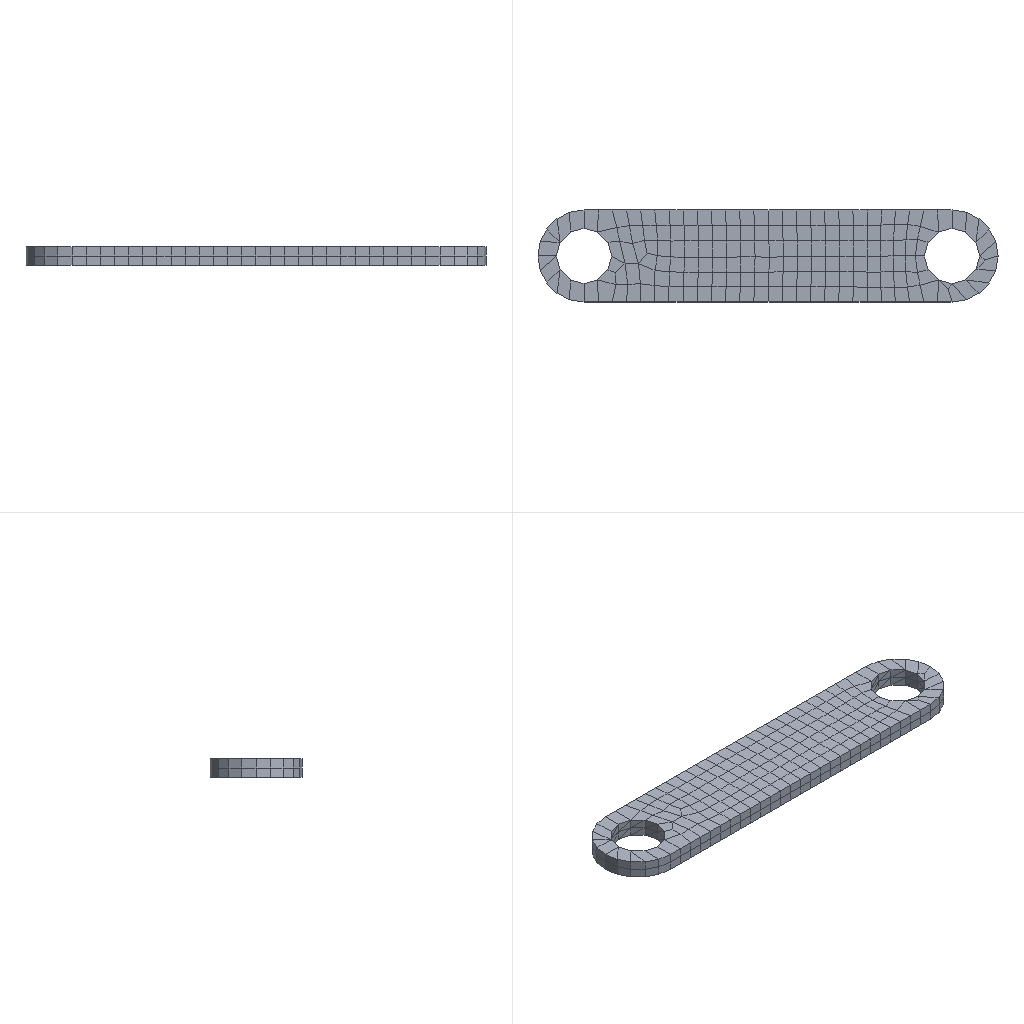Simulation study | ansys workbench
Set-up summary:
category,name,step,type,value,unit,region
solver,ansys_workbench
units,mm-N-s-tonne (MPa),,stated,"/units,MPA"
analysis,LS1,,transient
load_step,LS1,LS1,transient,nsubst=100; time=1
mesh,nodes,,,2205
mesh,elements,,,384
element_type,SOLID186,,,336
element_type,CONTA174,,,48
material,Structural Steel,,E,200000,tonne s^-2 mm^-1
material,Structural Steel,,nu,0.3
material,Structural Steel,,density,7.85e-09,tonne mm^-3
material,Structural Steel,,conductivity,60.5,tonne mm s^-3 C^-1
material,Structural Steel,,specific_heat,4.34e+08,mm^2 s^-2 C^-1
material,Structural Steel,,cte,1.2e-05,C^-1
material,Structural Steel,,permeability,10000
material,Structural Steel,,resistivity,0.00017,ohm mm
contact,contact 1,,bonded (always),element=CONTA174
contact,contact 2,,bonded (always),element=CONTA174
gap,no loads/excitations found in deck
Ansys APDL input file, long lists of numbers shortened:
/batch
/config,noeldb,1     ! force off writing results to database
*get,_wallstrt,active,,time,wall
! ANSYS input file written by Workbench version 2023 R2
! File used for geometry attach:
/title,wbnew--Transient (A5)
! ****** Begin Custom Load Command Snippet ******
/COM, ACT Extensions:
/COM,     LSDYNA, 2023.2
/COM,/COM,     ANSYSMotion, 2023.2
/COM,
! ****** End   Custom Load Command Snippet ******
*DIM,_wb_ProjectScratch_dir,string,248
_wb_ProjectScratch_dir(1) = ''
*DIM,_wb_SolverFiles_dir,string,248
_wb_SolverFiles_dir(1) = ''
*DIM,_wb_userfiles_dir,string,248
_wb_userfiles_dir(1) = ''
/com,--- Data in consistent NMM units. See Solving Units in the help system for more information.
/units,MPA
/nopr
/wb,file,start              !  signify a WB generated input file
/prep7
! Turn off shape checking because checks already performed inside WB mesher.
! See help system for more information.
SHPP,OFF,,NOWARN
/nolist
etcon,set             ! allow ANSYS to choose best KEYOP's for 180x elements, resets any applicable keyopt to MAPDL defaults
/com,*********** Nodes for the whole assembly ***********
nblock,3,,2416
(1i9,3e20.9e3)
        1    -2.448881254E+01     2.152807781E+00     1.630000025E+02
! (2196 more lines like these left out)
-1
/com,*********** Nodes for all Remote Points ***********
nblock,3
(1i9,3e20.9e3)
     2198    -3.448881218E+01     2.152807741E+00     1.630000025E+02
! (7 more lines like these left out)
-1
/wb,elem,start            !  set before creation of elements
/com,*********** Elements for Body 1 "crank" ***********
/com,*********** Send Body as a Rigid Body ***********
et,1,21
keyo,1,2,1             ! Moments of inertia in nodal coordinates
keyo,1,3,0         ! 3D Mass With Rotary Intertia
r,1,3.48526103262952e-006,3.48526103262952e-006,3.48526103262952e-006,3.29793436009623e-005,1.97766587972307e-004,2.28423576723811e-004
local,11,0,-24.489,2.153,163.,0.,0.,0.
nrot,1
csys,0
mat,1
real,1
type,1
en,865,1
/com,*********** Elements for Body 2 "rod" ***********
et,2,186
keyo,2,2,1          ! set full integration on SOLID186
eblock,19,solid,,336
(19i9)
        2        2        2        2        0        0        0        0       20        0        1        8      590      489      516      225      608      514      515
! (671 more lines like these left out)
-1
/com,*********** Elements for Body 3 "sliding" ***********
/com,*********** Send Body as a Rigid Body ***********
et,3,21
keyo,3,2,1             ! Moments of inertia in nodal coordinates
keyo,3,3,0         ! 3D Mass With Rotary Intertia
r,3,1.81689295804776e-006,1.81689295804776e-006,1.81689295804776e-006,2.6747344778675e-005,2.67473433929451e-005,5.22819186247149e-005
local,11,0,25.511,2.153,163.,0.,0.,0.
nrot,2197
csys,0
mat,3
real,3
type,3
en,866,2197
/wb,elem,end               !  done creating elements
/com,*********** Send User Defined Coordinate System(s) ***********
local,12,0,-34.489,2.153,163.,-180.,0.,-180.
local,13,0,-14.489,2.153,163.,-180.,0.,-180.
local,14,0,25.511,2.153,165.,0.,0.,0.
local,15,0,31.511,2.153,163.,0.,0.,0.
csys,0
toffst,273.15,  ! Temperature offset from absolute zero
/com,*********** Set Reference Temperature ***********
tref,22.
/wb,mat,start              !  starting to send materials
/com,*********** Send Materials ***********
Temperature = 'TEMP' ! Temperature
MP,DENS,1,7.85e-09,	! tonne mm^-3
MP,ALPX,1,1.2e-05,	! C^-1
MP,C,1,434000000,	! mm^2 s^-2 C^-1
MP,KXX,1,60.5,	! tonne mm s^-3 C^-1
MP,RSVX,1,0.00017,	! ohm mm
MP,EX,1,200000,	! tonne s^-2 mm^-1
MP,NUXY,1,0.3,
MP,MURX,1,10000,
Temperature = 'TEMP' ! Temperature
MP,DENS,2,7.85e-09,	! tonne mm^-3
MP,ALPX,2,1.2e-05,	! C^-1
MP,C,2,434000000,	! mm^2 s^-2 C^-1
MP,KXX,2,60.5,	! tonne mm s^-3 C^-1
MP,RSVX,2,0.00017,	! ohm mm
MP,EX,2,200000,	! tonne s^-2 mm^-1
MP,NUXY,2,0.3,
MP,MURX,2,10000,
Temperature = 'TEMP' ! Temperature
MP,DENS,3,7.85e-09,	! tonne mm^-3
MP,ALPX,3,1.2e-05,	! C^-1
MP,C,3,434000000,	! mm^2 s^-2 C^-1
MP,KXX,3,60.5,	! tonne mm s^-3 C^-1
MP,RSVX,3,0.00017,	! ohm mm
MP,EX,3,200000,	! tonne s^-2 mm^-1
MP,NUXY,3,0.3,
MP,MURX,3,10000,
/wb,mat,end                !  done sending materials
!************************* Model Summary ********************
!crank,	Structural Steel,	matid,	1
!rod,	Structural Steel,	matid,	2
!sliding,	Structural Steel,	matid,	3
!************************* End Model Summary ********************
! get the diagonal of the bounding box. Needed later for other things
*get,_xmin,node,,mnloc,x
*get,_ymin,node,,mnloc,y
*get,_zmin,node,,mnloc,z
*get,_xmax,node,,mxloc,x
*get,_ymax,node,,mxloc,y
*get,_zmax,node,,mxloc,z
_ASMDIAG=(_xmax-_xmin)*(_xmax-_xmin)+(_ymax-_ymin)*(_ymax-_ymin)+(_zmax-_zmin)*(_zmax-_zmin)
_ASMDIAG=SQRT(_ASMDIAG)
/wb,contact,start          !  starting to send contact
/wb,contact,end            !  done creating contacts
/golist
/wb,load,start             !  starting to send loads
/com,*********** Create Remote Point "Internal Remote Point 2" ***********
! -------- Remote Point Used by "Revolute - Ground To crank" --------
! ********* Create Contact to Connect To Rigid Body Mass Node ***********
*set,tid,4
*set,cid,4
et,tid,170
keyo,tid,2,1           ! Set MPC target element and not fix pilot
keyo,tid,4,0           ! Create CE's for all DOFs
type,tid
mat ,cid
real,cid
tshape,pilo
en,879,1
tshape
! ********* End of Create Contact to Connect To Rigid Body Mass Node ***********
*set,_npilot,2199
_npilot49=_npilot
mat,4
real,4
type,4
en,880,1,2199
csys,12
nrot,2199
csys,0
/com,*********** Create Remote Point "Internal Remote Point 3" ***********
! -------- Remote Point Used by "Revolute - crank To rod" --------
*set,_npilot,2200
_npilot55=_npilot
mat,4
real,4
type,4
en,881,1,2200
csys,13
nrot,2200
csys,0
/com,*********** Create Remote Point "Internal Remote Point 4" ***********
! -------- Remote Point Used by "Revolute - crank To rod" --------
*set,tid,6
*set,cid,5
et,cid,174
et,tid,170
keyo,tid,2,1               ! Don't fix the pilot node
keyo,tid,4,0               ! Activate all DOF's due to large deformation
keyo,cid,12,5              ! Bonded Contact
keyo,cid,4,2               ! Rigid CERIG style load
keyo,cid,2,2               ! MPC style contact
eblock,10,,,24
(15i9)
      882        5        5        5        0      611      623      347      357     2163     1647     1646     1679
! (23 more lines like these left out)
-1
*set,_npilot,2201
_npilot56=_npilot
type,tid
mat ,cid
real,cid
tshape,pilo
en,906,_npilot
tshape
csys,13
nrot,2201
csys,0
/com,*********** Create Remote Point "Internal Remote Point 5" ***********
! -------- Remote Point Used by "Revolute - rod To sliding" --------
*set,tid,8
*set,cid,7
et,cid,174
et,tid,170
keyo,tid,2,1               ! Don't fix the pilot node
keyo,tid,4,0               ! Activate all DOF's due to large deformation
keyo,cid,12,5              ! Bonded Contact
keyo,cid,4,2               ! Rigid CERIG style load
keyo,cid,2,2               ! MPC style contact
eblock,10,,,24
(15i9)
      907        7        7        7        0      587      599      359      369     2127     1685     1683     1713
! (23 more lines like these left out)
-1
*set,_npilot,2202
_npilot63=_npilot
type,tid
mat ,cid
real,cid
tshape,pilo
en,931,_npilot
tshape
/com,*********** Create Remote Point "Internal Remote Point 6" ***********
! -------- Remote Point Used by "Revolute - rod To sliding" --------
! ********* Create Contact to Connect To Rigid Body Mass Node ***********
*set,tid,9
*set,cid,9
et,tid,170
keyo,tid,2,1           ! Set MPC target element and not fix pilot
keyo,tid,4,0           ! Create CE's for all DOFs
type,tid
mat ,cid
real,cid
tshape,pilo
en,932,2197
tshape
! ********* End of Create Contact to Connect To Rigid Body Mass Node ***********
*set,_npilot,2203
_npilot64=_npilot
mat,9
real,9
type,9
en,933,2197,2203
/com,*********** Create Remote Point "Internal Remote Point 8" ***********
! -------- Remote Point Used by "Translational - Ground To sliding" --------
*set,_npilot,2205
_npilot72=_npilot
mat,9
real,9
type,9
en,934,2197,2205
/com,*********** Create Joint "Revolute - Ground To crank" ***********
/com,            Real Constant Set For Above Joint Is 10
! Joint Element Type Declaration and Definition using MPC184
*set,_jid,10
et,_jid,184
keyo,_jid,1,6           ! Revolute Joint
keyo,_jid,4,1           ! Z Axis is revolute axis
sectype,_jid, joint, revo, _wbjoint
secjoint,,12,12
mat,_jid
real,_jid
type,_jid
secnum,_jid
en,867,,2199        ! body to ground joint
/com,*********** Create Joint "Revolute - crank To rod" ***********
/com,            Real Constant Set For Above Joint Is 11
! Joint Element Type Declaration and Definition using MPC184
*set,_jid,11
et,_jid,184
keyo,_jid,1,6           ! Revolute Joint
keyo,_jid,4,1           ! Z Axis is revolute axis
sectype,_jid, joint, revo, _wbjoint
secjoint,,13,13
mat,_jid
real,_jid
type,_jid
secnum,_jid
en,868,2200,2201      ! body to body joint
/com,*********** Create Joint "Revolute - rod To sliding" ***********
/com,            Real Constant Set For Above Joint Is 12
! Joint Element Type Declaration and Definition using MPC184
*set,_jid,12
et,_jid,184
keyo,_jid,1,6           ! Revolute Joint
keyo,_jid,4,1           ! Z Axis is revolute axis
sectype,_jid, joint, revo, _wbjoint
secjoint,,14,14
mat,_jid
real,_jid
type,_jid
secnum,_jid
en,869,2202,2203      ! body to body joint
/com,*********** Create Joint "Translational - Ground To sliding" ***********
/com,            Real Constant Set For Above Joint Is 13
! Joint Element Type Declaration and Definition using MPC184
*set,_jid,13
et,_jid,184
keyo,_jid,1,10          ! Prismatic Joint
sectype,_jid, joint, pris, _wbjoint
secjoint,,15,15
mat,_jid
real,_jid
type,_jid
secnum,_jid
en,870,,2205        ! body to ground joint
/com,*********** Create Joint Drivers **********
*DIM,_loadvari78,TABLE,2,1,1,TIME
! Time values
*TAXIS,_loadvari78(1),1,0.,1.
! Load values
_loadvari78(1,1,1) = 10.
_loadvari78(2,1,1) = 10.
/gst,on,on
fini
*get,_numnode,node,0,count
*get,_numelem,elem,0,count
*get, _MAXELEMNUM, elem, 0, NUM, MAX
*get, _MAXNODENUM, node, 0, NUM, MAX
*get, _MAXELEMTYPE, etyp, 0, NUM, MAX
*get, _MAXREALCONST, rcon, 0, NUM, MAX
/go
/wb,load,end               !  done creating loads
/com,--- Number of total nodes = %_numnode%
/com,--- Number of contact elements = 48
/com,--- Number of spring elements = 0
/com,--- Number of bearing elements = 0
/com,--- Number of solid elements = 338
/com,--- Number of condensed parts = 0
/com,--- Number of total elements = %_numelem%
*get,_wallbsol,active,,time,wall
/com,****************************************************************************
/com,*************************    SOLUTION       ********************************
/com,****************************************************************************
/solu
antype,4                   ! transient analysis
nlgeom,on                  ! Turn on Large Deformation Effects
kbc,1                      ! stepped BC's
_thickRatio=  0     ! Ratio of thick parts in the model
eqsl,sparse,,,,,1
cntr,print,1               ! print out contact info and also make no initial contact an error
cncheck,dmp		!	Enable program controlled contact splitting for distributed memory parallel run
dmpoption,emat,no             ! Don't combine emat file for DANSYS
dmpoption,esav,no             ! Don't combine esav file for DANSYS
trnopt,full,,,,,hht        ! HHT time integration method
tintp, mosp			! Choose transient integration settings for moderate speed application
nldiag,cont,iter           ! print out contact info each equilibrium iteration
rescontrol,define,last,last,,dele	   ! Program Controlled
/com,****************************************************
/com,******************* SOLVE FOR LS 1 OF 1 ****************
/nopr
/gopr
esel,s,type,,10
dj,all,omgz,%_loadvari78%
esel,all
autots,off                 ! User turned off automatic time stepping
nsub,100,100,100
time,1.
timint,on                  ! Turn on time integration effects
outres,erase
outres,all,none
outres,nsol,all,
outres,rsol,all
outres,eangl,all
outres,etmp,all
outres,veng,all
outres,strs,all,
outres,epel,all,
outres,eppl,all,
outres,cont,all,
outres,v,all,
outres,a,all,
/nopr
esel,s,type,,1
esel,a,type,,3
esel,a,type,,10,13
cm,_elmisc,elem
esel,all
/gopr
outres,misc,all,_elmisc
! *********** WB SOLVE COMMAND ***********
! check interactive state
*get,ANSINTER_,active,,int
*if,ANSINTER_,ne,0,then
/eof
*endif
solve
/com *************** Write FE CONNECTORS *********
CEWRITE,file,ce,,INTE
/com,****************************************************
/com,*************** FINISHED SOLVE FOR LS 1 *************
*get,_wallasol,active,,time,wall
/nopr
*get,_numnode,node,0,count
*get,_numelem,elem,0,count
*get, _MAXELEMNUM, elem, 0, NUM, MAX
*get, _MAXNODENUM, node, 0, NUM, MAX,,,INTERNAL
*get, _MAXELEMTYPE, etyp, 0, NUM, MAX
*get, _MAXREALCONST, rcon, 0, NUM, MAX
*get,_NSOLTHREADS,active,0,ntfs
*get,_NSOLPROCESSES,active,0,npfs
/gopr
/post1
xmlo,ENCODING,ISO-8859-1
xmlo,parm
/xml,parm,xml
fini
/gopr
*get,_walldone,active,,time,wall
_preptime=(_wallbsol-_wallstrt)*3600
_solvtime=(_wallasol-_wallbsol)*3600
_posttime=(_walldone-_wallasol)*3600
_totaltim=(_walldone-_wallstrt)*3600
*get,_dlbratio,active,0,solu,dlbr
*get,_combtime,active,0,solu,comb
*get,_ssmode,active,0,solu,ssmm
*get,_ndofs,active,0,solu,ndof
*get,_sol_end_time,active,0,set,time
*if,_sol_end_time,eq,1.,then
/fclean				!clean distributed files
*endif
/com,--- Total number of nodes = %_numnode%
/com,--- Total number of elements = %_numelem%
/com,--- Element load balance ratio = %_dlbratio%
/com,--- Time to combine distributed files = %_combtime%
/com,--- Sparse memory mode = %_ssmode%
/com,--- Number of DOF = %_ndofs%
/wb,file,end               ! done with WB generated input
Results summary:
result,analyses[0].index,,,1
result,analyses[0].system,,,SYS
result,analyses[0].deck,,,deck.dat
result,analyses[0].solve_status,,,completed
result,analyses[0].analysis_type,,,static
result,analyses[0].physics,,,mechanical
result,analyses[0].unit_system,,,"NMM: mm, ton, N, s, mV, mA, degC"
result,analyses[0].n_sets,,,100
result,analyses[0].load_steps[0].set,set=100,,100
result,analyses[0].load_steps[0].time_or_freq,set=100,,1
result,analyses[0].load_steps[0].max_displacement_magnitude,set=100,,39.73
result,analyses[0].load_steps[0].max_von_mises_nodal,set=100,,0.0008984
result,analyses[0].load_steps[0].reaction_force_sum_xyz[1],set=100,,0
result,analyses[0].load_steps[0].reaction_force_sum_xyz[2],set=100,,0
result,analyses[0].load_steps[0].reaction_force_sum_xyz[3],set=100,,0
result,geometry_export[0][0],,,.step
result,geometry_export[0][1],,,ok
result,geometry_export[0][2],,,3